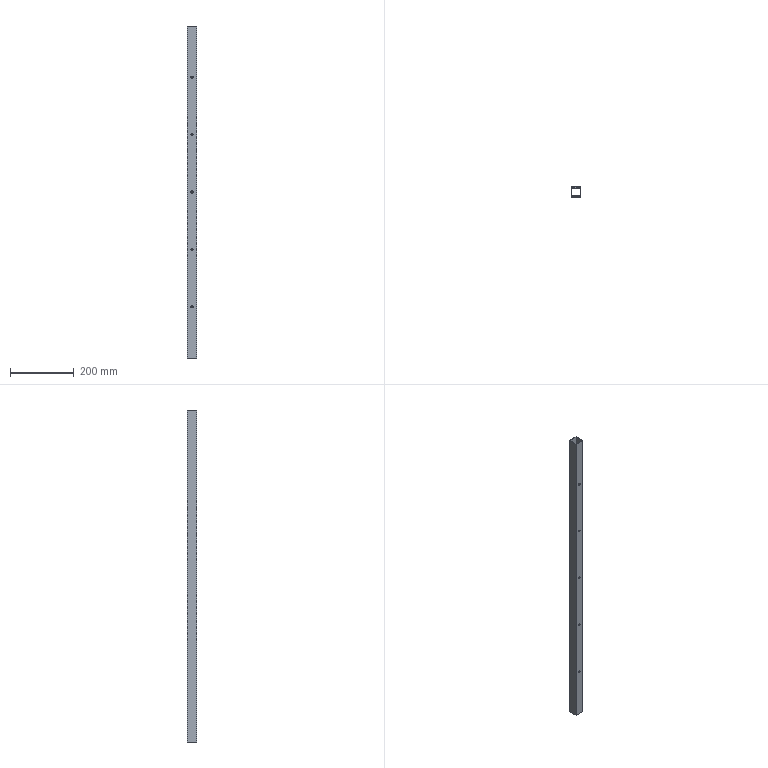Part | SolidWorks | features Extrusion 1, ICE 1 | 1 solid | 30 faces | box 30 x 30 x 1040 mm | volume 232276 mm3 | cylinder 20 | plane 10 | commonest cylinder face diameters 6.6 x20
STEP:
#1=CARTESIAN_POINT('',(0.,13.,-356.7));
#2=VERTEX_POINT('',#1);
#3=CARTESIAN_POINT('',(0.,13.,-363.3));
#4=VERTEX_POINT('',#3);
#5=CARTESIAN_POINT('',(0.,13.,-360.));
#6=DIRECTION('',(0.,-1.,0.));
#7=DIRECTION('',(0.,0.,-1.));
#8=AXIS2_PLACEMENT_3D('',#5,#6,#7);
#9=CIRCLE('',#8,3.3);
#10=EDGE_CURVE('',#2,#4,#9,.T.);
#11=ORIENTED_EDGE('',*,*,#10,.T.);
#12=CARTESIAN_POINT('',(0.,15.,-363.3));
#13=VERTEX_POINT('',#12);
#14=CARTESIAN_POINT('',(0.,-621.,-363.3));
#15=DIRECTION('',(0.,1.,0.));
#16=VECTOR('',#15,1000.);
#17=LINE('',#14,#16);
#18=EDGE_CURVE('',#4,#13,#17,.T.);
#19=ORIENTED_EDGE('',*,*,#18,.T.);
#20=CARTESIAN_POINT('',(0.,15.,-356.7));
#21=VERTEX_POINT('',#20);
#22=CARTESIAN_POINT('',(0.,15.,-360.));
#23=DIRECTION('',(0.,1.,0.));
#24=DIRECTION('',(0.,0.,1.));
#25=AXIS2_PLACEMENT_3D('',#22,#23,#24);
#26=CIRCLE('',#25,3.3);
#27=EDGE_CURVE('',#13,#21,#26,.T.);
#28=ORIENTED_EDGE('',*,*,#27,.T.);
#29=CARTESIAN_POINT('',(0.,-621.,-356.7));
#30=DIRECTION('',(0.,1.,0.));
#31=VECTOR('',#30,1000.);
#32=LINE('',#29,#31);
#33=EDGE_CURVE('',#2,#21,#32,.T.);
#34=ORIENTED_EDGE('',*,*,#33,.F.);
#35=EDGE_LOOP('',(#11,#19,#28,#34));
#36=FACE_OUTER_BOUND('',#35,.T.);
#37=CARTESIAN_POINT('',(0.,-621.,-360.));
#38=DIRECTION('',(0.,1.,0.));
#39=DIRECTION('',(0.,0.,1.));
#40=AXIS2_PLACEMENT_3D('',#37,#38,#39);
#41=CYLINDRICAL_SURFACE('',#40,3.3);
#42=ADVANCED_FACE('',(#36),#41,.F.);
#43=CARTESIAN_POINT('',(0.,13.,-176.7));
#44=VERTEX_POINT('',#43);
#45=CARTESIAN_POINT('',(0.,13.,-183.3));
#46=VERTEX_POINT('',#45);
#47=CARTESIAN_POINT('',(0.,13.,-180.));
#48=DIRECTION('',(0.,-1.,0.));
#49=DIRECTION('',(0.,0.,-1.));
#50=AXIS2_PLACEMENT_3D('',#47,#48,#49);
#51=CIRCLE('',#50,3.3);
#52=EDGE_CURVE('',#44,#46,#51,.T.);
#53=ORIENTED_EDGE('',*,*,#52,.T.);
#54=CARTESIAN_POINT('',(0.,15.,-183.3));
#55=VERTEX_POINT('',#54);
#56=CARTESIAN_POINT('',(0.,-621.,-183.3));
#57=DIRECTION('',(0.,1.,0.));
#58=VECTOR('',#57,1000.);
#59=LINE('',#56,#58);
#60=EDGE_CURVE('',#46,#55,#59,.T.);
#61=ORIENTED_EDGE('',*,*,#60,.T.);
#62=CARTESIAN_POINT('',(0.,15.,-176.7));
#63=VERTEX_POINT('',#62);
#64=CARTESIAN_POINT('',(0.,15.,-180.));
#65=DIRECTION('',(0.,1.,0.));
#66=DIRECTION('',(0.,0.,1.));
#67=AXIS2_PLACEMENT_3D('',#64,#65,#66);
#68=CIRCLE('',#67,3.3);
#69=EDGE_CURVE('',#55,#63,#68,.T.);
#70=ORIENTED_EDGE('',*,*,#69,.T.);
#71=CARTESIAN_POINT('',(0.,-621.,-176.7));
#72=DIRECTION('',(0.,1.,0.));
#73=VECTOR('',#72,1000.);
#74=LINE('',#71,#73);
#75=EDGE_CURVE('',#44,#63,#74,.T.);
#76=ORIENTED_EDGE('',*,*,#75,.F.);
#77=EDGE_LOOP('',(#53,#61,#70,#76));
#78=FACE_OUTER_BOUND('',#77,.T.);
#79=CARTESIAN_POINT('',(0.,-621.,-180.));
#80=DIRECTION('',(0.,1.,0.));
#81=DIRECTION('',(0.,0.,1.));
#82=AXIS2_PLACEMENT_3D('',#79,#80,#81);
#83=CYLINDRICAL_SURFACE('',#82,3.3);
#84=ADVANCED_FACE('',(#78),#83,.F.);
#85=CARTESIAN_POINT('',(0.,13.,3.3));
#86=VERTEX_POINT('',#85);
#87=CARTESIAN_POINT('',(0.,13.,-3.3));
#88=VERTEX_POINT('',#87);
#89=CARTESIAN_POINT('',(0.,13.,0.));
#90=DIRECTION('',(0.,-1.,0.));
#91=DIRECTION('',(0.,0.,-1.));
#92=AXIS2_PLACEMENT_3D('',#89,#90,#91);
#93=CIRCLE('',#92,3.3);
#94=EDGE_CURVE('',#86,#88,#93,.T.);
#95=ORIENTED_EDGE('',*,*,#94,.T.);
#96=CARTESIAN_POINT('',(0.,15.,-3.3));
#97=VERTEX_POINT('',#96);
#98=CARTESIAN_POINT('',(0.,-621.,-3.3));
#99=DIRECTION('',(0.,1.,0.));
#100=VECTOR('',#99,1000.);
#101=LINE('',#98,#100);
#102=EDGE_CURVE('',#88,#97,#101,.T.);
#103=ORIENTED_EDGE('',*,*,#102,.T.);
#104=CARTESIAN_POINT('',(0.,15.,3.3));
#105=VERTEX_POINT('',#104);
#106=CARTESIAN_POINT('',(0.,15.,0.));
#107=DIRECTION('',(0.,1.,0.));
#108=DIRECTION('',(0.,0.,1.));
#109=AXIS2_PLACEMENT_3D('',#106,#107,#108);
#110=CIRCLE('',#109,3.3);
#111=EDGE_CURVE('',#97,#105,#110,.T.);
#112=ORIENTED_EDGE('',*,*,#111,.T.);
#113=CARTESIAN_POINT('',(0.,-621.,3.3));
#114=DIRECTION('',(0.,1.,0.));
#115=VECTOR('',#114,1000.);
#116=LINE('',#113,#115);
#117=EDGE_CURVE('',#86,#105,#116,.T.);
#118=ORIENTED_EDGE('',*,*,#117,.F.);
#119=EDGE_LOOP('',(#95,#103,#112,#118));
#120=FACE_OUTER_BOUND('',#119,.T.);
#121=CARTESIAN_POINT('',(0.,-621.,0.));
#122=DIRECTION('',(0.,1.,0.));
#123=DIRECTION('',(0.,0.,1.));
#124=AXIS2_PLACEMENT_3D('',#121,#122,#123);
#125=CYLINDRICAL_SURFACE('',#124,3.3);
#126=ADVANCED_FACE('',(#120),#125,.F.);
#127=CARTESIAN_POINT('',(0.,13.,183.3));
#128=VERTEX_POINT('',#127);
#129=CARTESIAN_POINT('',(0.,13.,176.7));
#130=VERTEX_POINT('',#129);
#131=CARTESIAN_POINT('',(0.,13.,180.));
#132=DIRECTION('',(0.,-1.,0.));
#133=DIRECTION('',(0.,0.,-1.));
#134=AXIS2_PLACEMENT_3D('',#131,#132,#133);
#135=CIRCLE('',#134,3.3);
#136=EDGE_CURVE('',#128,#130,#135,.T.);
#137=ORIENTED_EDGE('',*,*,#136,.T.);
#138=CARTESIAN_POINT('',(0.,15.,176.7));
#139=VERTEX_POINT('',#138);
#140=CARTESIAN_POINT('',(0.,-621.,176.7));
#141=DIRECTION('',(0.,1.,0.));
#142=VECTOR('',#141,1000.);
#143=LINE('',#140,#142);
#144=EDGE_CURVE('',#130,#139,#143,.T.);
#145=ORIENTED_EDGE('',*,*,#144,.T.);
#146=CARTESIAN_POINT('',(0.,15.,183.3));
#147=VERTEX_POINT('',#146);
#148=CARTESIAN_POINT('',(0.,15.,180.));
#149=DIRECTION('',(0.,1.,0.));
#150=DIRECTION('',(0.,0.,1.));
#151=AXIS2_PLACEMENT_3D('',#148,#149,#150);
#152=CIRCLE('',#151,3.3);
#153=EDGE_CURVE('',#139,#147,#152,.T.);
#154=ORIENTED_EDGE('',*,*,#153,.T.);
#155=CARTESIAN_POINT('',(0.,-621.,183.3));
#156=DIRECTION('',(0.,1.,0.));
#157=VECTOR('',#156,1000.);
#158=LINE('',#155,#157);
#159=EDGE_CURVE('',#128,#147,#158,.T.);
#160=ORIENTED_EDGE('',*,*,#159,.F.);
#161=EDGE_LOOP('',(#137,#145,#154,#160));
#162=FACE_OUTER_BOUND('',#161,.T.);
#163=CARTESIAN_POINT('',(0.,-621.,180.));
#164=DIRECTION('',(0.,1.,0.));
#165=DIRECTION('',(0.,0.,1.));
#166=AXIS2_PLACEMENT_3D('',#163,#164,#165);
#167=CYLINDRICAL_SURFACE('',#166,3.3);
#168=ADVANCED_FACE('',(#162),#167,.F.);
#169=CARTESIAN_POINT('',(0.,13.,363.3));
#170=VERTEX_POINT('',#169);
#171=CARTESIAN_POINT('',(0.,13.,356.7));
#172=VERTEX_POINT('',#171);
#173=CARTESIAN_POINT('',(0.,13.,360.));
#174=DIRECTION('',(0.,-1.,0.));
#175=DIRECTION('',(0.,0.,-1.));
#176=AXIS2_PLACEMENT_3D('',#173,#174,#175);
#177=CIRCLE('',#176,3.3);
#178=EDGE_CURVE('',#170,#172,#177,.T.);
#179=ORIENTED_EDGE('',*,*,#178,.T.);
#180=CARTESIAN_POINT('',(0.,15.,356.7));
#181=VERTEX_POINT('',#180);
#182=CARTESIAN_POINT('',(0.,-621.,356.7));
#183=DIRECTION('',(0.,1.,0.));
#184=VECTOR('',#183,1000.);
#185=LINE('',#182,#184);
#186=EDGE_CURVE('',#172,#181,#185,.T.);
#187=ORIENTED_EDGE('',*,*,#186,.T.);
#188=CARTESIAN_POINT('',(0.,15.,363.3));
#189=VERTEX_POINT('',#188);
#190=CARTESIAN_POINT('',(0.,15.,360.));
#191=DIRECTION('',(0.,1.,0.));
#192=DIRECTION('',(0.,0.,1.));
#193=AXIS2_PLACEMENT_3D('',#190,#191,#192);
#194=CIRCLE('',#193,3.3);
#195=EDGE_CURVE('',#181,#189,#194,.T.);
#196=ORIENTED_EDGE('',*,*,#195,.T.);
#197=CARTESIAN_POINT('',(0.,-621.,363.3));
#198=DIRECTION('',(0.,1.,0.));
#199=VECTOR('',#198,1000.);
#200=LINE('',#197,#199);
#201=EDGE_CURVE('',#170,#189,#200,.T.);
#202=ORIENTED_EDGE('',*,*,#201,.F.);
#203=EDGE_LOOP('',(#179,#187,#196,#202));
#204=FACE_OUTER_BOUND('',#203,.T.);
#205=CARTESIAN_POINT('',(0.,-621.,360.));
#206=DIRECTION('',(0.,1.,0.));
#207=DIRECTION('',(0.,0.,1.));
#208=AXIS2_PLACEMENT_3D('',#205,#206,#207);
#209=CYLINDRICAL_SURFACE('',#208,3.3);
#210=ADVANCED_FACE('',(#204),#209,.F.);
#211=CARTESIAN_POINT('',(0.,-15.,-363.3));
#212=VERTEX_POINT('',#211);
#213=CARTESIAN_POINT('',(0.,-15.,-356.7));
#214=VERTEX_POINT('',#213);
#215=CARTESIAN_POINT('',(0.,-15.,-360.));
#216=DIRECTION('',(0.,1.,0.));
#217=DIRECTION('',(-1.,0.,0.));
#218=AXIS2_PLACEMENT_3D('',#215,#216,#217);
#219=CIRCLE('',#218,3.3);
#220=EDGE_CURVE('',#212,#214,#219,.T.);
#221=ORIENTED_EDGE('',*,*,#220,.F.);
#222=CARTESIAN_POINT('',(0.,-13.,-363.3));
#223=VERTEX_POINT('',#222);
#224=CARTESIAN_POINT('',(0.,-621.,-363.3));
#225=DIRECTION('',(0.,1.,0.));
#226=VECTOR('',#225,1000.);
#227=LINE('',#224,#226);
#228=EDGE_CURVE('',#212,#223,#227,.T.);
#229=ORIENTED_EDGE('',*,*,#228,.T.);
#230=CARTESIAN_POINT('',(0.,-13.,-356.7));
#231=VERTEX_POINT('',#230);
#232=CARTESIAN_POINT('',(0.,-13.,-360.));
#233=DIRECTION('',(0.,1.,0.));
#234=DIRECTION('',(0.,0.,1.));
#235=AXIS2_PLACEMENT_3D('',#232,#233,#234);
#236=CIRCLE('',#235,3.3);
#237=EDGE_CURVE('',#223,#231,#236,.T.);
#238=ORIENTED_EDGE('',*,*,#237,.T.);
#239=CARTESIAN_POINT('',(0.,-621.,-356.7));
#240=DIRECTION('',(0.,1.,0.));
#241=VECTOR('',#240,1000.);
#242=LINE('',#239,#241);
#243=EDGE_CURVE('',#214,#231,#242,.T.);
#244=ORIENTED_EDGE('',*,*,#243,.F.);
#245=EDGE_LOOP('',(#221,#229,#238,#244));
#246=FACE_OUTER_BOUND('',#245,.T.);
#247=CARTESIAN_POINT('',(0.,-621.,-360.));
#248=DIRECTION('',(0.,1.,0.));
#249=DIRECTION('',(0.,0.,1.));
#250=AXIS2_PLACEMENT_3D('',#247,#248,#249);
#251=CYLINDRICAL_SURFACE('',#250,3.3);
#252=ADVANCED_FACE('',(#246),#251,.F.);
#253=CARTESIAN_POINT('',(0.,-15.,-183.3));
#254=VERTEX_POINT('',#253);
#255=CARTESIAN_POINT('',(0.,-15.,-176.7));
#256=VERTEX_POINT('',#255);
#257=CARTESIAN_POINT('',(0.,-15.,-180.));
#258=DIRECTION('',(0.,1.,0.));
#259=DIRECTION('',(-1.,0.,0.));
#260=AXIS2_PLACEMENT_3D('',#257,#258,#259);
#261=CIRCLE('',#260,3.3);
#262=EDGE_CURVE('',#254,#256,#261,.T.);
#263=ORIENTED_EDGE('',*,*,#262,.F.);
#264=CARTESIAN_POINT('',(0.,-13.,-183.3));
#265=VERTEX_POINT('',#264);
#266=CARTESIAN_POINT('',(0.,-621.,-183.3));
#267=DIRECTION('',(0.,1.,0.));
#268=VECTOR('',#267,1000.);
#269=LINE('',#266,#268);
#270=EDGE_CURVE('',#254,#265,#269,.T.);
#271=ORIENTED_EDGE('',*,*,#270,.T.);
#272=CARTESIAN_POINT('',(0.,-13.,-176.7));
#273=VERTEX_POINT('',#272);
#274=CARTESIAN_POINT('',(0.,-13.,-180.));
#275=DIRECTION('',(0.,1.,0.));
#276=DIRECTION('',(0.,0.,1.));
#277=AXIS2_PLACEMENT_3D('',#274,#275,#276);
#278=CIRCLE('',#277,3.3);
#279=EDGE_CURVE('',#265,#273,#278,.T.);
#280=ORIENTED_EDGE('',*,*,#279,.T.);
#281=CARTESIAN_POINT('',(0.,-621.,-176.7));
#282=DIRECTION('',(0.,1.,0.));
#283=VECTOR('',#282,1000.);
#284=LINE('',#281,#283);
#285=EDGE_CURVE('',#256,#273,#284,.T.);
#286=ORIENTED_EDGE('',*,*,#285,.F.);
#287=EDGE_LOOP('',(#263,#271,#280,#286));
#288=FACE_OUTER_BOUND('',#287,.T.);
#289=CARTESIAN_POINT('',(0.,-621.,-180.));
#290=DIRECTION('',(0.,1.,0.));
#291=DIRECTION('',(0.,0.,1.));
#292=AXIS2_PLACEMENT_3D('',#289,#290,#291);
#293=CYLINDRICAL_SURFACE('',#292,3.3);
#294=ADVANCED_FACE('',(#288),#293,.F.);
#295=CARTESIAN_POINT('',(0.,-15.,-3.3));
#296=VERTEX_POINT('',#295);
#297=CARTESIAN_POINT('',(0.,-15.,3.3));
#298=VERTEX_POINT('',#297);
#299=CARTESIAN_POINT('',(0.,-15.,0.));
#300=DIRECTION('',(0.,1.,0.));
#301=DIRECTION('',(-1.,0.,0.));
#302=AXIS2_PLACEMENT_3D('',#299,#300,#301);
#303=CIRCLE('',#302,3.3);
#304=EDGE_CURVE('',#296,#298,#303,.T.);
#305=ORIENTED_EDGE('',*,*,#304,.F.);
#306=CARTESIAN_POINT('',(0.,-13.,-3.3));
#307=VERTEX_POINT('',#306);
#308=CARTESIAN_POINT('',(0.,-621.,-3.3));
#309=DIRECTION('',(0.,1.,0.));
#310=VECTOR('',#309,1000.);
#311=LINE('',#308,#310);
#312=EDGE_CURVE('',#296,#307,#311,.T.);
#313=ORIENTED_EDGE('',*,*,#312,.T.);
#314=CARTESIAN_POINT('',(0.,-13.,3.3));
#315=VERTEX_POINT('',#314);
#316=CARTESIAN_POINT('',(0.,-13.,0.));
#317=DIRECTION('',(0.,1.,0.));
#318=DIRECTION('',(0.,0.,1.));
#319=AXIS2_PLACEMENT_3D('',#316,#317,#318);
#320=CIRCLE('',#319,3.3);
#321=EDGE_CURVE('',#307,#315,#320,.T.);
#322=ORIENTED_EDGE('',*,*,#321,.T.);
#323=CARTESIAN_POINT('',(0.,-621.,3.3));
#324=DIRECTION('',(0.,1.,0.));
#325=VECTOR('',#324,1000.);
#326=LINE('',#323,#325);
#327=EDGE_CURVE('',#298,#315,#326,.T.);
#328=ORIENTED_EDGE('',*,*,#327,.F.);
#329=EDGE_LOOP('',(#305,#313,#322,#328));
#330=FACE_OUTER_BOUND('',#329,.T.);
#331=CARTESIAN_POINT('',(0.,-621.,0.));
#332=DIRECTION('',(0.,1.,0.));
#333=DIRECTION('',(0.,0.,1.));
#334=AXIS2_PLACEMENT_3D('',#331,#332,#333);
#335=CYLINDRICAL_SURFACE('',#334,3.3);
#336=ADVANCED_FACE('',(#330),#335,.F.);
#337=CARTESIAN_POINT('',(0.,-15.,176.7));
#338=VERTEX_POINT('',#337);
#339=CARTESIAN_POINT('',(0.,-15.,183.3));
#340=VERTEX_POINT('',#339);
#341=CARTESIAN_POINT('',(0.,-15.,180.));
#342=DIRECTION('',(0.,1.,0.));
#343=DIRECTION('',(-1.,0.,0.));
#344=AXIS2_PLACEMENT_3D('',#341,#342,#343);
#345=CIRCLE('',#344,3.3);
#346=EDGE_CURVE('',#338,#340,#345,.T.);
#347=ORIENTED_EDGE('',*,*,#346,.F.);
#348=CARTESIAN_POINT('',(0.,-13.,176.7));
#349=VERTEX_POINT('',#348);
#350=CARTESIAN_POINT('',(0.,-621.,176.7));
#351=DIRECTION('',(0.,1.,0.));
#352=VECTOR('',#351,1000.);
#353=LINE('',#350,#352);
#354=EDGE_CURVE('',#338,#349,#353,.T.);
#355=ORIENTED_EDGE('',*,*,#354,.T.);
#356=CARTESIAN_POINT('',(0.,-13.,183.3));
#357=VERTEX_POINT('',#356);
#358=CARTESIAN_POINT('',(0.,-13.,180.));
#359=DIRECTION('',(0.,1.,0.));
#360=DIRECTION('',(0.,0.,1.));
#361=AXIS2_PLACEMENT_3D('',#358,#359,#360);
#362=CIRCLE('',#361,3.3);
#363=EDGE_CURVE('',#349,#357,#362,.T.);
#364=ORIENTED_EDGE('',*,*,#363,.T.);
#365=CARTESIAN_POINT('',(0.,-621.,183.3));
#366=DIRECTION('',(0.,1.,0.));
#367=VECTOR('',#366,1000.);
#368=LINE('',#365,#367);
#369=EDGE_CURVE('',#340,#357,#368,.T.);
#370=ORIENTED_EDGE('',*,*,#369,.F.);
#371=EDGE_LOOP('',(#347,#355,#364,#370));
#372=FACE_OUTER_BOUND('',#371,.T.);
#373=CARTESIAN_POINT('',(0.,-621.,180.));
#374=DIRECTION('',(0.,1.,0.));
#375=DIRECTION('',(0.,0.,1.));
#376=AXIS2_PLACEMENT_3D('',#373,#374,#375);
#377=CYLINDRICAL_SURFACE('',#376,3.3);
#378=ADVANCED_FACE('',(#372),#377,.F.);
#379=CARTESIAN_POINT('',(0.,-15.,356.7));
#380=VERTEX_POINT('',#379);
#381=CARTESIAN_POINT('',(0.,-15.,363.3));
#382=VERTEX_POINT('',#381);
#383=CARTESIAN_POINT('',(0.,-15.,360.));
#384=DIRECTION('',(0.,1.,0.));
#385=DIRECTION('',(-1.,0.,0.));
#386=AXIS2_PLACEMENT_3D('',#383,#384,#385);
#387=CIRCLE('',#386,3.3);
#388=EDGE_CURVE('',#380,#382,#387,.T.);
#389=ORIENTED_EDGE('',*,*,#388,.F.);
#390=CARTESIAN_POINT('',(0.,-13.,356.7));
#391=VERTEX_POINT('',#390);
#392=CARTESIAN_POINT('',(0.,-621.,356.7));
#393=DIRECTION('',(0.,1.,0.));
#394=VECTOR('',#393,1000.);
#395=LINE('',#392,#394);
#396=EDGE_CURVE('',#380,#391,#395,.T.);
#397=ORIENTED_EDGE('',*,*,#396,.T.);
#398=CARTESIAN_POINT('',(0.,-13.,363.3));
#399=VERTEX_POINT('',#398);
#400=CARTESIAN_POINT('',(0.,-13.,360.));
#401=DIRECTION('',(0.,1.,0.));
#402=DIRECTION('',(0.,0.,1.));
#403=AXIS2_PLACEMENT_3D('',#400,#401,#402);
#404=CIRCLE('',#403,3.3);
#405=EDGE_CURVE('',#391,#399,#404,.T.);
#406=ORIENTED_EDGE('',*,*,#405,.T.);
#407=CARTESIAN_POINT('',(0.,-621.,363.3));
#408=DIRECTION('',(0.,1.,0.));
#409=VECTOR('',#408,1000.);
#410=LINE('',#407,#409);
#411=EDGE_CURVE('',#382,#399,#410,.T.);
#412=ORIENTED_EDGE('',*,*,#411,.F.);
#413=EDGE_LOOP('',(#389,#397,#406,#412));
#414=FACE_OUTER_BOUND('',#413,.T.);
#415=CARTESIAN_POINT('',(0.,-621.,360.));
#416=DIRECTION('',(0.,1.,0.));
#417=DIRECTION('',(0.,0.,1.));
#418=AXIS2_PLACEMENT_3D('',#415,#416,#417);
#419=CYLINDRICAL_SURFACE('',#418,3.3);
#420=ADVANCED_FACE('',(#414),#419,.F.);
#421=CARTESIAN_POINT('',(-15.,15.,520.));
#422=VERTEX_POINT('',#421);
#423=CARTESIAN_POINT('',(-15.,-15.,520.));
#424=VERTEX_POINT('',#423);
#425=CARTESIAN_POINT('',(-15.,-15.,520.));
#426=DIRECTION('',(0.,-1.,0.));
#427=VECTOR('',#426,1000.);
#428=LINE('',#425,#427);
#429=EDGE_CURVE('',#422,#424,#428,.T.);
#430=ORIENTED_EDGE('',*,*,#429,.T.);
#431=CARTESIAN_POINT('',(15.,-15.,520.));
#432=VERTEX_POINT('',#431);
#433=CARTESIAN_POINT('',(15.,-15.,520.));
#434=DIRECTION('',(1.,0.,0.));
#435=VECTOR('',#434,1000.);
#436=LINE('',#433,#435);
#437=EDGE_CURVE('',#424,#432,#436,.T.);
#438=ORIENTED_EDGE('',*,*,#437,.T.);
#439=CARTESIAN_POINT('',(15.,15.,520.));
#440=VERTEX_POINT('',#439);
#441=CARTESIAN_POINT('',(15.,-15.,520.));
#442=DIRECTION('',(0.,1.,0.));
#443=VECTOR('',#442,1000.);
#444=LINE('',#441,#443);
#445=EDGE_CURVE('',#432,#440,#444,.T.);
#446=ORIENTED_EDGE('',*,*,#445,.T.);
#447=CARTESIAN_POINT('',(15.,15.,520.));
#448=DIRECTION('',(-1.,0.,0.));
#449=VECTOR('',#448,1000.);
#450=LINE('',#447,#449);
#451=EDGE_CURVE('',#440,#422,#450,.T.);
#452=ORIENTED_EDGE('',*,*,#451,.T.);
#453=EDGE_LOOP('',(#430,#438,#446,#452));
#454=FACE_OUTER_BOUND('',#453,.T.);
#455=CARTESIAN_POINT('',(13.,13.,520.));
#456=VERTEX_POINT('',#455);
#457=CARTESIAN_POINT('',(-13.,13.,520.));
#458=VERTEX_POINT('',#457);
#459=CARTESIAN_POINT('',(13.,13.,520.));
#460=DIRECTION('',(-1.,0.,0.));
#461=VECTOR('',#460,1000.);
#462=LINE('',#459,#461);
#463=EDGE_CURVE('',#456,#458,#462,.T.);
#464=ORIENTED_EDGE('',*,*,#463,.F.);
#465=CARTESIAN_POINT('',(13.,-13.,520.));
#466=VERTEX_POINT('',#465);
#467=CARTESIAN_POINT('',(13.,-13.,520.));
#468=DIRECTION('',(0.,1.,0.));
#469=VECTOR('',#468,1000.);
#470=LINE('',#467,#469);
#471=EDGE_CURVE('',#466,#456,#470,.T.);
#472=ORIENTED_EDGE('',*,*,#471,.F.);
#473=CARTESIAN_POINT('',(-13.,-13.,520.));
#474=VERTEX_POINT('',#473);
#475=CARTESIAN_POINT('',(13.,-13.,520.));
#476=DIRECTION('',(1.,0.,0.));
#477=VECTOR('',#476,1000.);
#478=LINE('',#475,#477);
#479=EDGE_CURVE('',#474,#466,#478,.T.);
#480=ORIENTED_EDGE('',*,*,#479,.F.);
#481=CARTESIAN_POINT('',(-13.,-13.,520.));
#482=DIRECTION('',(0.,-1.,0.));
#483=VECTOR('',#482,1000.);
#484=LINE('',#481,#483);
#485=EDGE_CURVE('',#458,#474,#484,.T.);
#486=ORIENTED_EDGE('',*,*,#485,.F.);
#487=EDGE_LOOP('',(#464,#472,#480,#486));
#488=FACE_BOUND('',#487,.T.);
#489=CARTESIAN_POINT('',(0.,0.,520.));
#490=DIRECTION('',(0.,0.,1.));
#491=DIRECTION('',(1.,0.,0.));
#492=AXIS2_PLACEMENT_3D('',#489,#490,#491);
#493=PLANE('',#492);
#494=ADVANCED_FACE('',(#454,#488),#493,.T.);
#495=CARTESIAN_POINT('',(-15.,15.,-520.));
#496=VERTEX_POINT('',#495);
#497=CARTESIAN_POINT('',(-15.,-15.,-520.));
#498=VERTEX_POINT('',#497);
#499=CARTESIAN_POINT('',(-15.,-15.,-520.));
#500=DIRECTION('',(0.,-1.,0.));
#501=VECTOR('',#500,1000.);
#502=LINE('',#499,#501);
#503=EDGE_CURVE('',#496,#498,#502,.T.);
#504=ORIENTED_EDGE('',*,*,#503,.F.);
#505=CARTESIAN_POINT('',(15.,15.,-520.));
#506=VERTEX_POINT('',#505);
#507=CARTESIAN_POINT('',(15.,15.,-520.));
#508=DIRECTION('',(-1.,0.,0.));
#509=VECTOR('',#508,1000.);
#510=LINE('',#507,#509);
#511=EDGE_CURVE('',#506,#496,#510,.T.);
#512=ORIENTED_EDGE('',*,*,#511,.F.);
#513=CARTESIAN_POINT('',(15.,-15.,-520.));
#514=VERTEX_POINT('',#513);
#515=CARTESIAN_POINT('',(15.,-15.,-520.));
#516=DIRECTION('',(0.,1.,0.));
#517=VECTOR('',#516,1000.);
#518=LINE('',#515,#517);
#519=EDGE_CURVE('',#514,#506,#518,.T.);
#520=ORIENTED_EDGE('',*,*,#519,.F.);
#521=CARTESIAN_POINT('',(15.,-15.,-520.));
#522=DIRECTION('',(1.,0.,0.));
#523=VECTOR('',#522,1000.);
#524=LINE('',#521,#523);
#525=EDGE_CURVE('',#498,#514,#524,.T.);
#526=ORIENTED_EDGE('',*,*,#525,.F.);
#527=EDGE_LOOP('',(#504,#512,#520,#526));
#528=FACE_OUTER_BOUND('',#527,.T.);
#529=CARTESIAN_POINT('',(13.,-13.,-520.));
#530=VERTEX_POINT('',#529);
#531=CARTESIAN_POINT('',(13.,13.,-520.));
#532=VERTEX_POINT('',#531);
#533=CARTESIAN_POINT('',(13.,-13.,-520.));
#534=DIRECTION('',(0.,1.,0.));
#535=VECTOR('',#534,1000.);
#536=LINE('',#533,#535);
#537=EDGE_CURVE('',#530,#532,#536,.T.);
#538=ORIENTED_EDGE('',*,*,#537,.T.);
#539=CARTESIAN_POINT('',(-13.,13.,-520.));
#540=VERTEX_POINT('',#539);
#541=CARTESIAN_POINT('',(13.,13.,-520.));
#542=DIRECTION('',(-1.,0.,0.));
#543=VECTOR('',#542,1000.);
#544=LINE('',#541,#543);
#545=EDGE_CURVE('',#532,#540,#544,.T.);
#546=ORIENTED_EDGE('',*,*,#545,.T.);
#547=CARTESIAN_POINT('',(-13.,-13.,-520.));
#548=VERTEX_POINT('',#547);
#549=CARTESIAN_POINT('',(-13.,-13.,-520.));
#550=DIRECTION('',(0.,-1.,0.));
#551=VECTOR('',#550,1000.);
#552=LINE('',#549,#551);
#553=EDGE_CURVE('',#540,#548,#552,.T.);
#554=ORIENTED_EDGE('',*,*,#553,.T.);
#555=CARTESIAN_POINT('',(13.,-13.,-520.));
#556=DIRECTION('',(1.,0.,0.));
#557=VECTOR('',#556,1000.);
#558=LINE('',#555,#557);
#559=EDGE_CURVE('',#548,#530,#558,.T.);
#560=ORIENTED_EDGE('',*,*,#559,.T.);
#561=EDGE_LOOP('',(#538,#546,#554,#560));
#562=FACE_BOUND('',#561,.T.);
#563=CARTESIAN_POINT('',(0.,0.,-520.));
#564=DIRECTION('',(0.,0.,1.));
#565=DIRECTION('',(1.,0.,0.));
#566=AXIS2_PLACEMENT_3D('',#563,#564,#565);
#567=PLANE('',#566);
#568=ADVANCED_FACE('',(#528,#562),#567,.F.);
#569=ORIENTED_EDGE('',*,*,#503,.T.);
#570=CARTESIAN_POINT('',(-15.,-15.,520.));
#571=DIRECTION('',(0.,0.,-1.));
#572=VECTOR('',#571,1000.);
#573=LINE('',#570,#572);
#574=EDGE_CURVE('',#424,#498,#573,.T.);
#575=ORIENTED_EDGE('',*,*,#574,.F.);
#576=ORIENTED_EDGE('',*,*,#429,.F.);
#577=CARTESIAN_POINT('',(-15.,15.,520.));
#578=DIRECTION('',(0.,0.,-1.));
#579=VECTOR('',#578,1000.);
#580=LINE('',#577,#579);
#581=EDGE_CURVE('',#422,#496,#580,.T.);
#582=ORIENTED_EDGE('',*,*,#581,.T.);
#583=EDGE_LOOP('',(#569,#575,#576,#582));
#584=FACE_OUTER_BOUND('',#583,.T.);
#585=CARTESIAN_POINT('',(-15.,-15.,520.));
#586=DIRECTION('',(1.,0.,0.));
#587=DIRECTION('',(0.,1.,0.));
#588=AXIS2_PLACEMENT_3D('',#585,#586,#587);
#589=PLANE('',#588);
#590=ADVANCED_FACE('',(#584),#589,.F.);
#591=CARTESIAN_POINT('',(0.,-15.,-360.));
#592=DIRECTION('',(0.,1.,0.));
#593=DIRECTION('',(-1.,0.,0.));
#594=AXIS2_PLACEMENT_3D('',#591,#592,#593);
#595=CIRCLE('',#594,3.3);
#596=EDGE_CURVE('',#214,#212,#595,.T.);
#597=ORIENTED_EDGE('',*,*,#596,.T.);
#598=ORIENTED_EDGE('',*,*,#220,.T.);
#599=EDGE_LOOP('',(#597,#598));
#600=FACE_BOUND('',#599,.T.);
#601=CARTESIAN_POINT('',(0.,-15.,-180.));
#602=DIRECTION('',(0.,1.,0.));
#603=DIRECTION('',(-1.,0.,0.));
#604=AXIS2_PLACEMENT_3D('',#601,#602,#603);
#605=CIRCLE('',#604,3.3);
#606=EDGE_CURVE('',#256,#254,#605,.T.);
#607=ORIENTED_EDGE('',*,*,#606,.T.);
#608=ORIENTED_EDGE('',*,*,#262,.T.);
#609=EDGE_LOOP('',(#607,#608));
#610=FACE_BOUND('',#609,.T.);
#611=CARTESIAN_POINT('',(0.,-15.,0.));
#612=DIRECTION('',(0.,1.,0.));
#613=DIRECTION('',(-1.,0.,0.));
#614=AXIS2_PLACEMENT_3D('',#611,#612,#613);
#615=CIRCLE('',#614,3.3);
#616=EDGE_CURVE('',#298,#296,#615,.T.);
#617=ORIENTED_EDGE('',*,*,#616,.T.);
#618=ORIENTED_EDGE('',*,*,#304,.T.);
#619=EDGE_LOOP('',(#617,#618));
#620=FACE_BOUND('',#619,.T.);
#621=CARTESIAN_POINT('',(0.,-15.,180.));
#622=DIRECTION('',(0.,1.,0.));
#623=DIRECTION('',(-1.,0.,0.));
#624=AXIS2_PLACEMENT_3D('',#621,#622,#623);
#625=CIRCLE('',#624,3.3);
#626=EDGE_CURVE('',#340,#338,#625,.T.);
#627=ORIENTED_EDGE('',*,*,#626,.T.);
#628=ORIENTED_EDGE('',*,*,#346,.T.);
#629=EDGE_LOOP('',(#627,#628));
#630=FACE_BOUND('',#629,.T.);
#631=CARTESIAN_POINT('',(0.,-15.,360.));
#632=DIRECTION('',(0.,1.,0.));
#633=DIRECTION('',(-1.,0.,0.));
#634=AXIS2_PLACEMENT_3D('',#631,#632,#633);
#635=CIRCLE('',#634,3.3);
#636=EDGE_CURVE('',#382,#380,#635,.T.);
#637=ORIENTED_EDGE('',*,*,#636,.T.);
#638=ORIENTED_EDGE('',*,*,#388,.T.);
#639=EDGE_LOOP('',(#637,#638));
#640=FACE_BOUND('',#639,.T.);
#641=ORIENTED_EDGE('',*,*,#525,.T.);
#642=CARTESIAN_POINT('',(15.,-15.,520.));
#643=DIRECTION('',(0.,0.,-1.));
#644=VECTOR('',#643,1000.);
#645=LINE('',#642,#644);
#646=EDGE_CURVE('',#432,#514,#645,.T.);
#647=ORIENTED_EDGE('',*,*,#646,.F.);
#648=ORIENTED_EDGE('',*,*,#437,.F.);
#649=ORIENTED_EDGE('',*,*,#574,.T.);
#650=EDGE_LOOP('',(#641,#647,#648,#649));
#651=FACE_OUTER_BOUND('',#650,.T.);
#652=CARTESIAN_POINT('',(15.,-15.,520.));
#653=DIRECTION('',(0.,1.,0.));
#654=DIRECTION('',(-1.,0.,0.));
#655=AXIS2_PLACEMENT_3D('',#652,#653,#654);
#656=PLANE('',#655);
#657=ADVANCED_FACE('',(#600,#610,#620,#630,#640,#651),#656,.F.);
#658=ORIENTED_EDGE('',*,*,#519,.T.);
#659=CARTESIAN_POINT('',(15.,15.,520.));
#660=DIRECTION('',(0.,0.,-1.));
#661=VECTOR('',#660,1000.);
#662=LINE('',#659,#661);
#663=EDGE_CURVE('',#440,#506,#662,.T.);
#664=ORIENTED_EDGE('',*,*,#663,.F.);
#665=ORIENTED_EDGE('',*,*,#445,.F.);
#666=ORIENTED_EDGE('',*,*,#646,.T.);
#667=EDGE_LOOP('',(#658,#664,#665,#666));
#668=FACE_OUTER_BOUND('',#667,.T.);
#669=CARTESIAN_POINT('',(15.,-15.,520.));
#670=DIRECTION('',(-1.,0.,0.));
#671=DIRECTION('',(0.,0.,1.));
#672=AXIS2_PLACEMENT_3D('',#669,#670,#671);
#673=PLANE('',#672);
#674=ADVANCED_FACE('',(#668),#673,.F.);
#675=CARTESIAN_POINT('',(0.,15.,-360.));
#676=DIRECTION('',(0.,1.,0.));
#677=DIRECTION('',(0.,0.,1.));
#678=AXIS2_PLACEMENT_3D('',#675,#676,#677);
#679=CIRCLE('',#678,3.3);
#680=EDGE_CURVE('',#21,#13,#679,.T.);
#681=ORIENTED_EDGE('',*,*,#680,.F.);
#682=ORIENTED_EDGE('',*,*,#27,.F.);
#683=EDGE_LOOP('',(#681,#682));
#684=FACE_BOUND('',#683,.T.);
#685=CARTESIAN_POINT('',(0.,15.,-180.));
#686=DIRECTION('',(0.,1.,0.));
#687=DIRECTION('',(0.,0.,1.));
#688=AXIS2_PLACEMENT_3D('',#685,#686,#687);
#689=CIRCLE('',#688,3.3);
#690=EDGE_CURVE('',#63,#55,#689,.T.);
#691=ORIENTED_EDGE('',*,*,#690,.F.);
#692=ORIENTED_EDGE('',*,*,#69,.F.);
#693=EDGE_LOOP('',(#691,#692));
#694=FACE_BOUND('',#693,.T.);
#695=CARTESIAN_POINT('',(0.,15.,0.));
#696=DIRECTION('',(0.,1.,0.));
#697=DIRECTION('',(0.,0.,1.));
#698=AXIS2_PLACEMENT_3D('',#695,#696,#697);
#699=CIRCLE('',#698,3.3);
#700=EDGE_CURVE('',#105,#97,#699,.T.);
#701=ORIENTED_EDGE('',*,*,#700,.F.);
#702=ORIENTED_EDGE('',*,*,#111,.F.);
#703=EDGE_LOOP('',(#701,#702));
#704=FACE_BOUND('',#703,.T.);
#705=CARTESIAN_POINT('',(0.,15.,180.));
#706=DIRECTION('',(0.,1.,0.));
#707=DIRECTION('',(0.,0.,1.));
#708=AXIS2_PLACEMENT_3D('',#705,#706,#707);
#709=CIRCLE('',#708,3.3);
#710=EDGE_CURVE('',#147,#139,#709,.T.);
#711=ORIENTED_EDGE('',*,*,#710,.F.);
#712=ORIENTED_EDGE('',*,*,#153,.F.);
#713=EDGE_LOOP('',(#711,#712));
#714=FACE_BOUND('',#713,.T.);
#715=CARTESIAN_POINT('',(0.,15.,360.));
#716=DIRECTION('',(0.,1.,0.));
#717=DIRECTION('',(0.,0.,1.));
#718=AXIS2_PLACEMENT_3D('',#715,#716,#717);
#719=CIRCLE('',#718,3.3);
#720=EDGE_CURVE('',#189,#181,#719,.T.);
#721=ORIENTED_EDGE('',*,*,#720,.F.);
#722=ORIENTED_EDGE('',*,*,#195,.F.);
#723=EDGE_LOOP('',(#721,#722));
#724=FACE_BOUND('',#723,.T.);
#725=ORIENTED_EDGE('',*,*,#511,.T.);
#726=ORIENTED_EDGE('',*,*,#581,.F.);
#727=ORIENTED_EDGE('',*,*,#451,.F.);
#728=ORIENTED_EDGE('',*,*,#663,.T.);
#729=EDGE_LOOP('',(#725,#726,#727,#728));
#730=FACE_OUTER_BOUND('',#729,.T.);
#731=CARTESIAN_POINT('',(15.,15.,520.));
#732=DIRECTION('',(0.,-1.,0.));
#733=DIRECTION('',(0.,0.,-1.));
#734=AXIS2_PLACEMENT_3D('',#731,#732,#733);
#735=PLANE('',#734);
#736=ADVANCED_FACE('',(#684,#694,#704,#714,#724,#730),#735,.F.);
#737=ORIENTED_EDGE('',*,*,#537,.F.);
#738=CARTESIAN_POINT('',(13.,-13.,520.));
#739=DIRECTION('',(0.,0.,-1.));
#740=VECTOR('',#739,1000.);
#741=LINE('',#738,#740);
#742=EDGE_CURVE('',#466,#530,#741,.T.);
#743=ORIENTED_EDGE('',*,*,#742,.F.);
#744=ORIENTED_EDGE('',*,*,#471,.T.);
#745=CARTESIAN_POINT('',(13.,13.,520.));
#746=DIRECTION('',(0.,0.,-1.));
#747=VECTOR('',#746,1000.);
#748=LINE('',#745,#747);
#749=EDGE_CURVE('',#456,#532,#748,.T.);
#750=ORIENTED_EDGE('',*,*,#749,.T.);
#751=EDGE_LOOP('',(#737,#743,#744,#750));
#752=FACE_OUTER_BOUND('',#751,.T.);
#753=CARTESIAN_POINT('',(13.,-13.,520.));
#754=DIRECTION('',(-1.,0.,0.));
#755=DIRECTION('',(0.,0.,1.));
#756=AXIS2_PLACEMENT_3D('',#753,#754,#755);
#757=PLANE('',#756);
#758=ADVANCED_FACE('',(#752),#757,.T.);
#759=ORIENTED_EDGE('',*,*,#10,.F.);
#760=CARTESIAN_POINT('',(0.,13.,-360.));
#761=DIRECTION('',(0.,-1.,0.));
#762=DIRECTION('',(0.,0.,-1.));
#763=AXIS2_PLACEMENT_3D('',#760,#761,#762);
#764=CIRCLE('',#763,3.3);
#765=EDGE_CURVE('',#4,#2,#764,.T.);
#766=ORIENTED_EDGE('',*,*,#765,.F.);
#767=EDGE_LOOP('',(#759,#766));
#768=FACE_BOUND('',#767,.T.);
#769=ORIENTED_EDGE('',*,*,#52,.F.);
#770=CARTESIAN_POINT('',(0.,13.,-180.));
#771=DIRECTION('',(0.,-1.,0.));
#772=DIRECTION('',(0.,0.,-1.));
#773=AXIS2_PLACEMENT_3D('',#770,#771,#772);
#774=CIRCLE('',#773,3.3);
#775=EDGE_CURVE('',#46,#44,#774,.T.);
#776=ORIENTED_EDGE('',*,*,#775,.F.);
#777=EDGE_LOOP('',(#769,#776));
#778=FACE_BOUND('',#777,.T.);
#779=ORIENTED_EDGE('',*,*,#94,.F.);
#780=CARTESIAN_POINT('',(0.,13.,0.));
#781=DIRECTION('',(0.,-1.,0.));
#782=DIRECTION('',(0.,0.,-1.));
#783=AXIS2_PLACEMENT_3D('',#780,#781,#782);
#784=CIRCLE('',#783,3.3);
#785=EDGE_CURVE('',#88,#86,#784,.T.);
#786=ORIENTED_EDGE('',*,*,#785,.F.);
#787=EDGE_LOOP('',(#779,#786));
#788=FACE_BOUND('',#787,.T.);
#789=ORIENTED_EDGE('',*,*,#136,.F.);
#790=CARTESIAN_POINT('',(0.,13.,180.));
#791=DIRECTION('',(0.,-1.,0.));
#792=DIRECTION('',(0.,0.,-1.));
#793=AXIS2_PLACEMENT_3D('',#790,#791,#792);
#794=CIRCLE('',#793,3.3);
#795=EDGE_CURVE('',#130,#128,#794,.T.);
#796=ORIENTED_EDGE('',*,*,#795,.F.);
#797=EDGE_LOOP('',(#789,#796));
#798=FACE_BOUND('',#797,.T.);
#799=ORIENTED_EDGE('',*,*,#178,.F.);
#800=CARTESIAN_POINT('',(0.,13.,360.));
#801=DIRECTION('',(0.,-1.,0.));
#802=DIRECTION('',(0.,0.,-1.));
#803=AXIS2_PLACEMENT_3D('',#800,#801,#802);
#804=CIRCLE('',#803,3.3);
#805=EDGE_CURVE('',#172,#170,#804,.T.);
#806=ORIENTED_EDGE('',*,*,#805,.F.);
#807=EDGE_LOOP('',(#799,#806));
#808=FACE_BOUND('',#807,.T.);
#809=ORIENTED_EDGE('',*,*,#545,.F.);
#810=ORIENTED_EDGE('',*,*,#749,.F.);
#811=ORIENTED_EDGE('',*,*,#463,.T.);
#812=CARTESIAN_POINT('',(-13.,13.,520.));
#813=DIRECTION('',(0.,0.,-1.));
#814=VECTOR('',#813,1000.);
#815=LINE('',#812,#814);
#816=EDGE_CURVE('',#458,#540,#815,.T.);
#817=ORIENTED_EDGE('',*,*,#816,.T.);
#818=EDGE_LOOP('',(#809,#810,#811,#817));
#819=FACE_OUTER_BOUND('',#818,.T.);
#820=CARTESIAN_POINT('',(13.,13.,520.));
#821=DIRECTION('',(0.,-1.,0.));
#822=DIRECTION('',(0.,0.,-1.));
#823=AXIS2_PLACEMENT_3D('',#820,#821,#822);
#824=PLANE('',#823);
#825=ADVANCED_FACE('',(#768,#778,#788,#798,#808,#819),#824,.T.);
#826=ORIENTED_EDGE('',*,*,#553,.F.);
#827=ORIENTED_EDGE('',*,*,#816,.F.);
#828=ORIENTED_EDGE('',*,*,#485,.T.);
#829=CARTESIAN_POINT('',(-13.,-13.,520.));
#830=DIRECTION('',(0.,0.,-1.));
#831=VECTOR('',#830,1000.);
#832=LINE('',#829,#831);
#833=EDGE_CURVE('',#474,#548,#832,.T.);
#834=ORIENTED_EDGE('',*,*,#833,.T.);
#835=EDGE_LOOP('',(#826,#827,#828,#834));
#836=FACE_OUTER_BOUND('',#835,.T.);
#837=CARTESIAN_POINT('',(-13.,-13.,520.));
#838=DIRECTION('',(1.,0.,0.));
#839=DIRECTION('',(0.,0.,-1.));
#840=AXIS2_PLACEMENT_3D('',#837,#838,#839);
#841=PLANE('',#840);
#842=ADVANCED_FACE('',(#836),#841,.T.);
#843=CARTESIAN_POINT('',(0.,-13.,-360.));
#844=DIRECTION('',(0.,1.,0.));
#845=DIRECTION('',(0.,0.,1.));
#846=AXIS2_PLACEMENT_3D('',#843,#844,#845);
#847=CIRCLE('',#846,3.3);
#848=EDGE_CURVE('',#231,#223,#847,.T.);
#849=ORIENTED_EDGE('',*,*,#848,.F.);
#850=ORIENTED_EDGE('',*,*,#237,.F.);
#851=EDGE_LOOP('',(#849,#850));
#852=FACE_BOUND('',#851,.T.);
#853=CARTESIAN_POINT('',(0.,-13.,-180.));
#854=DIRECTION('',(0.,1.,0.));
#855=DIRECTION('',(0.,0.,1.));
#856=AXIS2_PLACEMENT_3D('',#853,#854,#855);
#857=CIRCLE('',#856,3.3);
#858=EDGE_CURVE('',#273,#265,#857,.T.);
#859=ORIENTED_EDGE('',*,*,#858,.F.);
#860=ORIENTED_EDGE('',*,*,#279,.F.);
#861=EDGE_LOOP('',(#859,#860));
#862=FACE_BOUND('',#861,.T.);
#863=CARTESIAN_POINT('',(0.,-13.,0.));
#864=DIRECTION('',(0.,1.,0.));
#865=DIRECTION('',(0.,0.,1.));
#866=AXIS2_PLACEMENT_3D('',#863,#864,#865);
#867=CIRCLE('',#866,3.3);
#868=EDGE_CURVE('',#315,#307,#867,.T.);
#869=ORIENTED_EDGE('',*,*,#868,.F.);
#870=ORIENTED_EDGE('',*,*,#321,.F.);
#871=EDGE_LOOP('',(#869,#870));
#872=FACE_BOUND('',#871,.T.);
#873=CARTESIAN_POINT('',(0.,-13.,180.));
#874=DIRECTION('',(0.,1.,0.));
#875=DIRECTION('',(0.,0.,1.));
#876=AXIS2_PLACEMENT_3D('',#873,#874,#875);
#877=CIRCLE('',#876,3.3);
#878=EDGE_CURVE('',#357,#349,#877,.T.);
#879=ORIENTED_EDGE('',*,*,#878,.F.);
#880=ORIENTED_EDGE('',*,*,#363,.F.);
#881=EDGE_LOOP('',(#879,#880));
#882=FACE_BOUND('',#881,.T.);
#883=CARTESIAN_POINT('',(0.,-13.,360.));
#884=DIRECTION('',(0.,1.,0.));
#885=DIRECTION('',(0.,0.,1.));
#886=AXIS2_PLACEMENT_3D('',#883,#884,#885);
#887=CIRCLE('',#886,3.3);
#888=EDGE_CURVE('',#399,#391,#887,.T.);
#889=ORIENTED_EDGE('',*,*,#888,.F.);
#890=ORIENTED_EDGE('',*,*,#405,.F.);
#891=EDGE_LOOP('',(#889,#890));
#892=FACE_BOUND('',#891,.T.);
#893=ORIENTED_EDGE('',*,*,#559,.F.);
#894=ORIENTED_EDGE('',*,*,#833,.F.);
#895=ORIENTED_EDGE('',*,*,#479,.T.);
#896=ORIENTED_EDGE('',*,*,#742,.T.);
#897=EDGE_LOOP('',(#893,#894,#895,#896));
#898=FACE_OUTER_BOUND('',#897,.T.);
#899=CARTESIAN_POINT('',(13.,-13.,520.));
#900=DIRECTION('',(0.,1.,0.));
#901=DIRECTION('',(0.,0.,1.));
#902=AXIS2_PLACEMENT_3D('',#899,#900,#901);
#903=PLANE('',#902);
#904=ADVANCED_FACE('',(#852,#862,#872,#882,#892,#898),#903,.T.);
#905=ORIENTED_EDGE('',*,*,#396,.F.);
#906=ORIENTED_EDGE('',*,*,#636,.F.);
#907=ORIENTED_EDGE('',*,*,#411,.T.);
#908=ORIENTED_EDGE('',*,*,#888,.T.);
#909=EDGE_LOOP('',(#905,#906,#907,#908));
#910=FACE_OUTER_BOUND('',#909,.T.);
#911=CARTESIAN_POINT('',(0.,-621.,360.));
#912=DIRECTION('',(0.,1.,0.));
#913=DIRECTION('',(0.,0.,1.));
#914=AXIS2_PLACEMENT_3D('',#911,#912,#913);
#915=CYLINDRICAL_SURFACE('',#914,3.3);
#916=ADVANCED_FACE('',(#910),#915,.F.);
#917=ORIENTED_EDGE('',*,*,#354,.F.);
#918=ORIENTED_EDGE('',*,*,#626,.F.);
#919=ORIENTED_EDGE('',*,*,#369,.T.);
#920=ORIENTED_EDGE('',*,*,#878,.T.);
#921=EDGE_LOOP('',(#917,#918,#919,#920));
#922=FACE_OUTER_BOUND('',#921,.T.);
#923=CARTESIAN_POINT('',(0.,-621.,180.));
#924=DIRECTION('',(0.,1.,0.));
#925=DIRECTION('',(0.,0.,1.));
#926=AXIS2_PLACEMENT_3D('',#923,#924,#925);
#927=CYLINDRICAL_SURFACE('',#926,3.3);
#928=ADVANCED_FACE('',(#922),#927,.F.);
#929=ORIENTED_EDGE('',*,*,#312,.F.);
#930=ORIENTED_EDGE('',*,*,#616,.F.);
#931=ORIENTED_EDGE('',*,*,#327,.T.);
#932=ORIENTED_EDGE('',*,*,#868,.T.);
#933=EDGE_LOOP('',(#929,#930,#931,#932));
#934=FACE_OUTER_BOUND('',#933,.T.);
#935=CARTESIAN_POINT('',(0.,-621.,0.));
#936=DIRECTION('',(0.,1.,0.));
#937=DIRECTION('',(0.,0.,1.));
#938=AXIS2_PLACEMENT_3D('',#935,#936,#937);
#939=CYLINDRICAL_SURFACE('',#938,3.3);
#940=ADVANCED_FACE('',(#934),#939,.F.);
#941=ORIENTED_EDGE('',*,*,#270,.F.);
#942=ORIENTED_EDGE('',*,*,#606,.F.);
#943=ORIENTED_EDGE('',*,*,#285,.T.);
#944=ORIENTED_EDGE('',*,*,#858,.T.);
#945=EDGE_LOOP('',(#941,#942,#943,#944));
#946=FACE_OUTER_BOUND('',#945,.T.);
#947=CARTESIAN_POINT('',(0.,-621.,-180.));
#948=DIRECTION('',(0.,1.,0.));
#949=DIRECTION('',(0.,0.,1.));
#950=AXIS2_PLACEMENT_3D('',#947,#948,#949);
#951=CYLINDRICAL_SURFACE('',#950,3.3);
#952=ADVANCED_FACE('',(#946),#951,.F.);
#953=ORIENTED_EDGE('',*,*,#228,.F.);
#954=ORIENTED_EDGE('',*,*,#596,.F.);
#955=ORIENTED_EDGE('',*,*,#243,.T.);
#956=ORIENTED_EDGE('',*,*,#848,.T.);
#957=EDGE_LOOP('',(#953,#954,#955,#956));
#958=FACE_OUTER_BOUND('',#957,.T.);
#959=CARTESIAN_POINT('',(0.,-621.,-360.));
#960=DIRECTION('',(0.,1.,0.));
#961=DIRECTION('',(0.,0.,1.));
#962=AXIS2_PLACEMENT_3D('',#959,#960,#961);
#963=CYLINDRICAL_SURFACE('',#962,3.3);
#964=ADVANCED_FACE('',(#958),#963,.F.);
#965=ORIENTED_EDGE('',*,*,#186,.F.);
#966=ORIENTED_EDGE('',*,*,#805,.T.);
#967=ORIENTED_EDGE('',*,*,#201,.T.);
#968=ORIENTED_EDGE('',*,*,#720,.T.);
#969=EDGE_LOOP('',(#965,#966,#967,#968));
#970=FACE_OUTER_BOUND('',#969,.T.);
#971=CARTESIAN_POINT('',(0.,-621.,360.));
#972=DIRECTION('',(0.,1.,0.));
#973=DIRECTION('',(0.,0.,1.));
#974=AXIS2_PLACEMENT_3D('',#971,#972,#973);
#975=CYLINDRICAL_SURFACE('',#974,3.3);
#976=ADVANCED_FACE('',(#970),#975,.F.);
#977=ORIENTED_EDGE('',*,*,#144,.F.);
#978=ORIENTED_EDGE('',*,*,#795,.T.);
#979=ORIENTED_EDGE('',*,*,#159,.T.);
#980=ORIENTED_EDGE('',*,*,#710,.T.);
#981=EDGE_LOOP('',(#977,#978,#979,#980));
#982=FACE_OUTER_BOUND('',#981,.T.);
#983=CARTESIAN_POINT('',(0.,-621.,180.));
#984=DIRECTION('',(0.,1.,0.));
#985=DIRECTION('',(0.,0.,1.));
#986=AXIS2_PLACEMENT_3D('',#983,#984,#985);
#987=CYLINDRICAL_SURFACE('',#986,3.3);
#988=ADVANCED_FACE('',(#982),#987,.F.);
#989=ORIENTED_EDGE('',*,*,#102,.F.);
#990=ORIENTED_EDGE('',*,*,#785,.T.);
#991=ORIENTED_EDGE('',*,*,#117,.T.);
#992=ORIENTED_EDGE('',*,*,#700,.T.);
#993=EDGE_LOOP('',(#989,#990,#991,#992));
#994=FACE_OUTER_BOUND('',#993,.T.);
#995=CARTESIAN_POINT('',(0.,-621.,0.));
#996=DIRECTION('',(0.,1.,0.));
#997=DIRECTION('',(0.,0.,1.));
#998=AXIS2_PLACEMENT_3D('',#995,#996,#997);
#999=CYLINDRICAL_SURFACE('',#998,3.3);
#1000=ADVANCED_FACE('',(#994),#999,.F.);
#1001=ORIENTED_EDGE('',*,*,#60,.F.);
#1002=ORIENTED_EDGE('',*,*,#775,.T.);
#1003=ORIENTED_EDGE('',*,*,#75,.T.);
#1004=ORIENTED_EDGE('',*,*,#690,.T.);
#1005=EDGE_LOOP('',(#1001,#1002,#1003,#1004));
#1006=FACE_OUTER_BOUND('',#1005,.T.);
#1007=CARTESIAN_POINT('',(0.,-621.,-180.));
#1008=DIRECTION('',(0.,1.,0.));
#1009=DIRECTION('',(0.,0.,1.));
#1010=AXIS2_PLACEMENT_3D('',#1007,#1008,#1009);
#1011=CYLINDRICAL_SURFACE('',#1010,3.3);
#1012=ADVANCED_FACE('',(#1006),#1011,.F.);
#1013=ORIENTED_EDGE('',*,*,#18,.F.);
#1014=ORIENTED_EDGE('',*,*,#765,.T.);
#1015=ORIENTED_EDGE('',*,*,#33,.T.);
#1016=ORIENTED_EDGE('',*,*,#680,.T.);
#1017=EDGE_LOOP('',(#1013,#1014,#1015,#1016));
#1018=FACE_OUTER_BOUND('',#1017,.T.);
#1019=CARTESIAN_POINT('',(0.,-621.,-360.));
#1020=DIRECTION('',(0.,1.,0.));
#1021=DIRECTION('',(0.,0.,1.));
#1022=AXIS2_PLACEMENT_3D('',#1019,#1020,#1021);
#1023=CYLINDRICAL_SURFACE('',#1022,3.3);
#1024=ADVANCED_FACE('',(#1018),#1023,.F.);
#1025=CLOSED_SHELL('',(#42,#84,#126,#168,#210,#252,#294,#336,#378,#420,#494,#568,#590,#657,#674,#736,#758,#825,#842,#904,#916,#928,#940,#952,#964,#976,#988,#1000,#1012,#1024));
#1026=MANIFOLD_SOLID_BREP('',#1025);
#1027=CARTESIAN_POINT('',(0.,0.,0.));
#1028=DIRECTION('',(0.,0.,1.));
#1029=DIRECTION('',(1.,0.,0.));
#1030=AXIS2_PLACEMENT_3D('',#1027,#1028,#1029);
#1031=(LENGTH_UNIT()NAMED_UNIT(*)SI_UNIT(.MILLI.,.METRE.));
#1032=UNCERTAINTY_MEASURE_WITH_UNIT(LENGTH_MEASURE(0.00001),#1031,'','');
#1033=(NAMED_UNIT(*)PLANE_ANGLE_UNIT()SI_UNIT($,.RADIAN.));
#1034=(NAMED_UNIT(*)SI_UNIT($,.STERADIAN.)SOLID_ANGLE_UNIT());
#1035=(GEOMETRIC_REPRESENTATION_CONTEXT(3)GLOBAL_UNCERTAINTY_ASSIGNED_CONTEXT((#1032))GLOBAL_UNIT_ASSIGNED_CONTEXT((#1031,#1033,#1034))REPRESENTATION_CONTEXT('',''));
#1036=ADVANCED_BREP_SHAPE_REPRESENTATION('',(#1026,#1030),#1035);